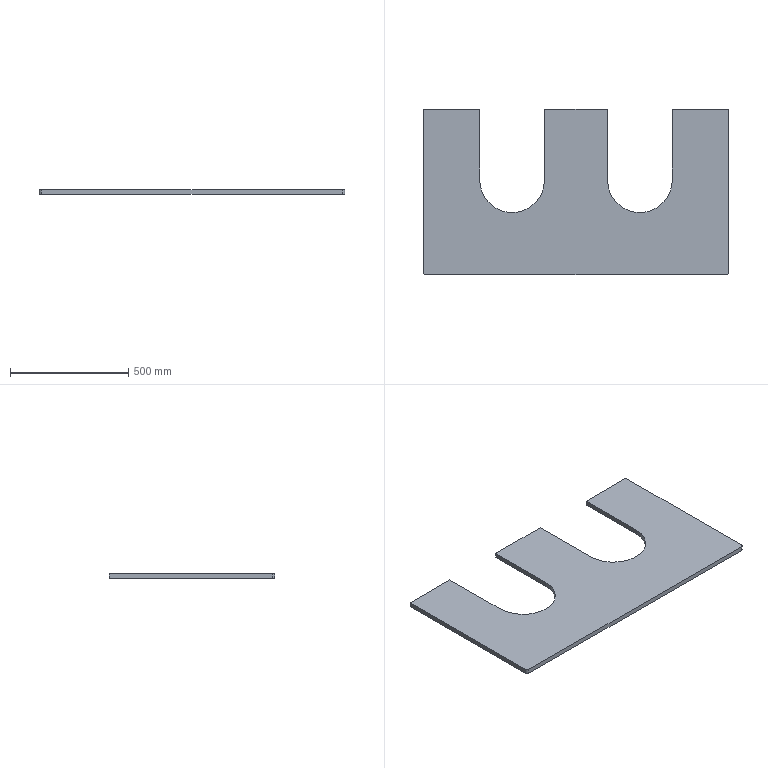Part | SolidWorks | features Extrusion 1, Fillet 1, ICE 1 | 1 solid | 16 faces | box 1290 x 700 x 20 mm | volume 13591851 mm3 | plane 12 | cylinder 4 | commonest cylinder face diameters 20 x2 274 x2
STEP:
#1=CARTESIAN_POINT('',(-407.,350.,20.));
#2=VERTEX_POINT('',#1);
#3=CARTESIAN_POINT('',(-645.,350.,20.));
#4=VERTEX_POINT('',#3);
#5=CARTESIAN_POINT('',(645.,350.,20.));
#6=DIRECTION('',(-1.,0.,0.));
#7=VECTOR('',#6,1000.);
#8=LINE('',#5,#7);
#9=EDGE_CURVE('',#2,#4,#8,.T.);
#10=ORIENTED_EDGE('',*,*,#9,.F.);
#11=CARTESIAN_POINT('',(-407.,350.,0.));
#12=VERTEX_POINT('',#11);
#13=CARTESIAN_POINT('',(-407.,350.,0.));
#14=DIRECTION('',(0.,0.,1.));
#15=VECTOR('',#14,1000.);
#16=LINE('',#13,#15);
#17=EDGE_CURVE('',#12,#2,#16,.T.);
#18=ORIENTED_EDGE('',*,*,#17,.F.);
#19=CARTESIAN_POINT('',(-645.,350.,0.));
#20=VERTEX_POINT('',#19);
#21=CARTESIAN_POINT('',(645.,350.,0.));
#22=DIRECTION('',(-1.,0.,0.));
#23=VECTOR('',#22,1000.);
#24=LINE('',#21,#23);
#25=EDGE_CURVE('',#12,#20,#24,.T.);
#26=ORIENTED_EDGE('',*,*,#25,.T.);
#27=CARTESIAN_POINT('',(-645.,350.,20.));
#28=DIRECTION('',(0.,0.,-1.));
#29=VECTOR('',#28,1000.);
#30=LINE('',#27,#29);
#31=EDGE_CURVE('',#4,#20,#30,.T.);
#32=ORIENTED_EDGE('',*,*,#31,.F.);
#33=EDGE_LOOP('',(#10,#18,#26,#32));
#34=FACE_OUTER_BOUND('',#33,.T.);
#35=CARTESIAN_POINT('',(645.,350.,20.));
#36=DIRECTION('',(0.,-1.,0.));
#37=DIRECTION('',(0.,0.,-1.));
#38=AXIS2_PLACEMENT_3D('',#35,#36,#37);
#39=PLANE('',#38);
#40=ADVANCED_FACE('',(#34),#39,.F.);
#41=CARTESIAN_POINT('',(133.,350.,0.));
#42=VERTEX_POINT('',#41);
#43=CARTESIAN_POINT('',(-133.,350.,0.));
#44=VERTEX_POINT('',#43);
#45=CARTESIAN_POINT('',(645.,350.,0.));
#46=DIRECTION('',(-1.,0.,0.));
#47=VECTOR('',#46,1000.);
#48=LINE('',#45,#47);
#49=EDGE_CURVE('',#42,#44,#48,.T.);
#50=ORIENTED_EDGE('',*,*,#49,.T.);
#51=CARTESIAN_POINT('',(-133.,350.,20.));
#52=VERTEX_POINT('',#51);
#53=CARTESIAN_POINT('',(-133.,350.,0.));
#54=DIRECTION('',(0.,0.,1.));
#55=VECTOR('',#54,1000.);
#56=LINE('',#53,#55);
#57=EDGE_CURVE('',#44,#52,#56,.T.);
#58=ORIENTED_EDGE('',*,*,#57,.T.);
#59=CARTESIAN_POINT('',(133.,350.,20.));
#60=VERTEX_POINT('',#59);
#61=CARTESIAN_POINT('',(645.,350.,20.));
#62=DIRECTION('',(-1.,0.,0.));
#63=VECTOR('',#62,1000.);
#64=LINE('',#61,#63);
#65=EDGE_CURVE('',#60,#52,#64,.T.);
#66=ORIENTED_EDGE('',*,*,#65,.F.);
#67=CARTESIAN_POINT('',(133.,350.,0.));
#68=DIRECTION('',(0.,0.,1.));
#69=VECTOR('',#68,1000.);
#70=LINE('',#67,#69);
#71=EDGE_CURVE('',#42,#60,#70,.T.);
#72=ORIENTED_EDGE('',*,*,#71,.F.);
#73=EDGE_LOOP('',(#50,#58,#66,#72));
#74=FACE_OUTER_BOUND('',#73,.T.);
#75=CARTESIAN_POINT('',(645.,350.,20.));
#76=DIRECTION('',(0.,-1.,0.));
#77=DIRECTION('',(0.,0.,-1.));
#78=AXIS2_PLACEMENT_3D('',#75,#76,#77);
#79=PLANE('',#78);
#80=ADVANCED_FACE('',(#74),#79,.F.);
#81=CARTESIAN_POINT('',(-645.,-340.,0.));
#82=VERTEX_POINT('',#81);
#83=CARTESIAN_POINT('',(-645.,-350.,0.));
#84=DIRECTION('',(0.,-1.,0.));
#85=VECTOR('',#84,1000.);
#86=LINE('',#83,#85);
#87=EDGE_CURVE('',#20,#82,#86,.T.);
#88=ORIENTED_EDGE('',*,*,#87,.T.);
#89=CARTESIAN_POINT('',(-645.,-340.,20.));
#90=VERTEX_POINT('',#89);
#91=CARTESIAN_POINT('',(-645.,-340.,20.));
#92=DIRECTION('',(0.,0.,1.));
#93=VECTOR('',#92,1000.);
#94=LINE('',#91,#93);
#95=EDGE_CURVE('',#82,#90,#94,.T.);
#96=ORIENTED_EDGE('',*,*,#95,.T.);
#97=CARTESIAN_POINT('',(-645.,-350.,20.));
#98=DIRECTION('',(0.,-1.,0.));
#99=VECTOR('',#98,1000.);
#100=LINE('',#97,#99);
#101=EDGE_CURVE('',#4,#90,#100,.T.);
#102=ORIENTED_EDGE('',*,*,#101,.F.);
#103=ORIENTED_EDGE('',*,*,#31,.T.);
#104=EDGE_LOOP('',(#88,#96,#102,#103));
#105=FACE_OUTER_BOUND('',#104,.T.);
#106=CARTESIAN_POINT('',(-645.,-350.,20.));
#107=DIRECTION('',(1.,0.,0.));
#108=DIRECTION('',(0.,0.,-1.));
#109=AXIS2_PLACEMENT_3D('',#106,#107,#108);
#110=PLANE('',#109);
#111=ADVANCED_FACE('',(#105),#110,.F.);
#112=CARTESIAN_POINT('',(-635.,-350.,0.));
#113=VERTEX_POINT('',#112);
#114=CARTESIAN_POINT('',(635.,-350.,0.));
#115=VERTEX_POINT('',#114);
#116=CARTESIAN_POINT('',(645.,-350.,0.));
#117=DIRECTION('',(1.,0.,0.));
#118=VECTOR('',#117,1000.);
#119=LINE('',#116,#118);
#120=EDGE_CURVE('',#113,#115,#119,.T.);
#121=ORIENTED_EDGE('',*,*,#120,.T.);
#122=CARTESIAN_POINT('',(635.,-350.,20.));
#123=VERTEX_POINT('',#122);
#124=CARTESIAN_POINT('',(635.,-350.,20.));
#125=DIRECTION('',(0.,0.,1.));
#126=VECTOR('',#125,1000.);
#127=LINE('',#124,#126);
#128=EDGE_CURVE('',#115,#123,#127,.T.);
#129=ORIENTED_EDGE('',*,*,#128,.T.);
#130=CARTESIAN_POINT('',(-635.,-350.,20.));
#131=VERTEX_POINT('',#130);
#132=CARTESIAN_POINT('',(645.,-350.,20.));
#133=DIRECTION('',(1.,0.,0.));
#134=VECTOR('',#133,1000.);
#135=LINE('',#132,#134);
#136=EDGE_CURVE('',#131,#123,#135,.T.);
#137=ORIENTED_EDGE('',*,*,#136,.F.);
#138=CARTESIAN_POINT('',(-635.,-350.,20.));
#139=DIRECTION('',(0.,0.,-1.));
#140=VECTOR('',#139,1000.);
#141=LINE('',#138,#140);
#142=EDGE_CURVE('',#131,#113,#141,.T.);
#143=ORIENTED_EDGE('',*,*,#142,.T.);
#144=EDGE_LOOP('',(#121,#129,#137,#143));
#145=FACE_OUTER_BOUND('',#144,.T.);
#146=CARTESIAN_POINT('',(645.,-350.,20.));
#147=DIRECTION('',(0.,1.,0.));
#148=DIRECTION('',(0.,0.,1.));
#149=AXIS2_PLACEMENT_3D('',#146,#147,#148);
#150=PLANE('',#149);
#151=ADVANCED_FACE('',(#145),#150,.F.);
#152=CARTESIAN_POINT('',(645.,-340.,20.));
#153=VERTEX_POINT('',#152);
#154=CARTESIAN_POINT('',(645.,350.,20.));
#155=VERTEX_POINT('',#154);
#156=CARTESIAN_POINT('',(645.,-350.,20.));
#157=DIRECTION('',(0.,1.,0.));
#158=VECTOR('',#157,1000.);
#159=LINE('',#156,#158);
#160=EDGE_CURVE('',#153,#155,#159,.T.);
#161=ORIENTED_EDGE('',*,*,#160,.F.);
#162=CARTESIAN_POINT('',(645.,-340.,0.));
#163=VERTEX_POINT('',#162);
#164=CARTESIAN_POINT('',(645.,-340.,20.));
#165=DIRECTION('',(0.,0.,-1.));
#166=VECTOR('',#165,1000.);
#167=LINE('',#164,#166);
#168=EDGE_CURVE('',#153,#163,#167,.T.);
#169=ORIENTED_EDGE('',*,*,#168,.T.);
#170=CARTESIAN_POINT('',(645.,350.,0.));
#171=VERTEX_POINT('',#170);
#172=CARTESIAN_POINT('',(645.,-350.,0.));
#173=DIRECTION('',(0.,1.,0.));
#174=VECTOR('',#173,1000.);
#175=LINE('',#172,#174);
#176=EDGE_CURVE('',#163,#171,#175,.T.);
#177=ORIENTED_EDGE('',*,*,#176,.T.);
#178=CARTESIAN_POINT('',(645.,350.,20.));
#179=DIRECTION('',(0.,0.,-1.));
#180=VECTOR('',#179,1000.);
#181=LINE('',#178,#180);
#182=EDGE_CURVE('',#155,#171,#181,.T.);
#183=ORIENTED_EDGE('',*,*,#182,.F.);
#184=EDGE_LOOP('',(#161,#169,#177,#183));
#185=FACE_OUTER_BOUND('',#184,.T.);
#186=CARTESIAN_POINT('',(645.,-350.,20.));
#187=DIRECTION('',(-1.,0.,0.));
#188=DIRECTION('',(0.,0.,1.));
#189=AXIS2_PLACEMENT_3D('',#186,#187,#188);
#190=PLANE('',#189);
#191=ADVANCED_FACE('',(#185),#190,.F.);
#192=CARTESIAN_POINT('',(407.,350.,0.));
#193=VERTEX_POINT('',#192);
#194=CARTESIAN_POINT('',(645.,350.,0.));
#195=DIRECTION('',(-1.,0.,0.));
#196=VECTOR('',#195,1000.);
#197=LINE('',#194,#196);
#198=EDGE_CURVE('',#171,#193,#197,.T.);
#199=ORIENTED_EDGE('',*,*,#198,.T.);
#200=CARTESIAN_POINT('',(407.,350.,20.));
#201=VERTEX_POINT('',#200);
#202=CARTESIAN_POINT('',(407.,350.,0.));
#203=DIRECTION('',(0.,0.,1.));
#204=VECTOR('',#203,1000.);
#205=LINE('',#202,#204);
#206=EDGE_CURVE('',#193,#201,#205,.T.);
#207=ORIENTED_EDGE('',*,*,#206,.T.);
#208=CARTESIAN_POINT('',(645.,350.,20.));
#209=DIRECTION('',(-1.,0.,0.));
#210=VECTOR('',#209,1000.);
#211=LINE('',#208,#210);
#212=EDGE_CURVE('',#155,#201,#211,.T.);
#213=ORIENTED_EDGE('',*,*,#212,.F.);
#214=ORIENTED_EDGE('',*,*,#182,.T.);
#215=EDGE_LOOP('',(#199,#207,#213,#214));
#216=FACE_OUTER_BOUND('',#215,.T.);
#217=CARTESIAN_POINT('',(645.,350.,20.));
#218=DIRECTION('',(0.,-1.,0.));
#219=DIRECTION('',(0.,0.,-1.));
#220=AXIS2_PLACEMENT_3D('',#217,#218,#219);
#221=PLANE('',#220);
#222=ADVANCED_FACE('',(#216),#221,.F.);
#223=ORIENTED_EDGE('',*,*,#136,.T.);
#224=CARTESIAN_POINT('',(635.,-340.,20.));
#225=DIRECTION('',(0.,0.,1.));
#226=DIRECTION('',(1.,0.,0.));
#227=AXIS2_PLACEMENT_3D('',#224,#225,#226);
#228=CIRCLE('',#227,10.);
#229=EDGE_CURVE('',#123,#153,#228,.T.);
#230=ORIENTED_EDGE('',*,*,#229,.T.);
#231=ORIENTED_EDGE('',*,*,#160,.T.);
#232=ORIENTED_EDGE('',*,*,#212,.T.);
#233=CARTESIAN_POINT('',(407.,50.,20.));
#234=VERTEX_POINT('',#233);
#235=CARTESIAN_POINT('',(407.,50.,20.));
#236=DIRECTION('',(0.,1.,0.));
#237=VECTOR('',#236,1000.);
#238=LINE('',#235,#237);
#239=EDGE_CURVE('',#234,#201,#238,.T.);
#240=ORIENTED_EDGE('',*,*,#239,.F.);
#241=CARTESIAN_POINT('',(133.,50.,20.));
#242=VERTEX_POINT('',#241);
#243=CARTESIAN_POINT('',(270.,50.,20.));
#244=DIRECTION('',(0.,0.,1.));
#245=DIRECTION('',(-1.,0.,0.));
#246=AXIS2_PLACEMENT_3D('',#243,#244,#245);
#247=CIRCLE('',#246,137.);
#248=EDGE_CURVE('',#242,#234,#247,.T.);
#249=ORIENTED_EDGE('',*,*,#248,.F.);
#250=CARTESIAN_POINT('',(133.,50.,20.));
#251=DIRECTION('',(0.,-1.,0.));
#252=VECTOR('',#251,1000.);
#253=LINE('',#250,#252);
#254=EDGE_CURVE('',#60,#242,#253,.T.);
#255=ORIENTED_EDGE('',*,*,#254,.F.);
#256=ORIENTED_EDGE('',*,*,#65,.T.);
#257=CARTESIAN_POINT('',(-133.,50.,20.));
#258=VERTEX_POINT('',#257);
#259=CARTESIAN_POINT('',(-133.,50.,20.));
#260=DIRECTION('',(0.,1.,0.));
#261=VECTOR('',#260,1000.);
#262=LINE('',#259,#261);
#263=EDGE_CURVE('',#258,#52,#262,.T.);
#264=ORIENTED_EDGE('',*,*,#263,.F.);
#265=CARTESIAN_POINT('',(-407.,50.,20.));
#266=VERTEX_POINT('',#265);
#267=CARTESIAN_POINT('',(-270.,50.,20.));
#268=DIRECTION('',(0.,0.,1.));
#269=DIRECTION('',(1.,0.,0.));
#270=AXIS2_PLACEMENT_3D('',#267,#268,#269);
#271=CIRCLE('',#270,137.);
#272=EDGE_CURVE('',#266,#258,#271,.T.);
#273=ORIENTED_EDGE('',*,*,#272,.F.);
#274=CARTESIAN_POINT('',(-407.,50.,20.));
#275=DIRECTION('',(0.,-1.,0.));
#276=VECTOR('',#275,1000.);
#277=LINE('',#274,#276);
#278=EDGE_CURVE('',#2,#266,#277,.T.);
#279=ORIENTED_EDGE('',*,*,#278,.F.);
#280=ORIENTED_EDGE('',*,*,#9,.T.);
#281=ORIENTED_EDGE('',*,*,#101,.T.);
#282=CARTESIAN_POINT('',(-635.,-340.,20.));
#283=DIRECTION('',(0.,0.,1.));
#284=DIRECTION('',(1.,0.,0.));
#285=AXIS2_PLACEMENT_3D('',#282,#283,#284);
#286=CIRCLE('',#285,10.);
#287=EDGE_CURVE('',#90,#131,#286,.T.);
#288=ORIENTED_EDGE('',*,*,#287,.T.);
#289=EDGE_LOOP('',(#223,#230,#231,#232,#240,#249,#255,#256,#264,#273,#279,#280,#281,#288));
#290=FACE_OUTER_BOUND('',#289,.T.);
#291=CARTESIAN_POINT('',(0.,0.,20.));
#292=DIRECTION('',(0.,0.,1.));
#293=DIRECTION('',(1.,0.,0.));
#294=AXIS2_PLACEMENT_3D('',#291,#292,#293);
#295=PLANE('',#294);
#296=ADVANCED_FACE('',(#290),#295,.T.);
#297=ORIENTED_EDGE('',*,*,#176,.F.);
#298=CARTESIAN_POINT('',(635.,-340.,0.));
#299=DIRECTION('',(0.,0.,-1.));
#300=DIRECTION('',(1.,0.,0.));
#301=AXIS2_PLACEMENT_3D('',#298,#299,#300);
#302=CIRCLE('',#301,10.);
#303=EDGE_CURVE('',#163,#115,#302,.T.);
#304=ORIENTED_EDGE('',*,*,#303,.T.);
#305=ORIENTED_EDGE('',*,*,#120,.F.);
#306=CARTESIAN_POINT('',(-635.,-340.,0.));
#307=DIRECTION('',(0.,0.,-1.));
#308=DIRECTION('',(1.,0.,0.));
#309=AXIS2_PLACEMENT_3D('',#306,#307,#308);
#310=CIRCLE('',#309,10.);
#311=EDGE_CURVE('',#113,#82,#310,.T.);
#312=ORIENTED_EDGE('',*,*,#311,.T.);
#313=ORIENTED_EDGE('',*,*,#87,.F.);
#314=ORIENTED_EDGE('',*,*,#25,.F.);
#315=CARTESIAN_POINT('',(-407.,50.,0.));
#316=VERTEX_POINT('',#315);
#317=CARTESIAN_POINT('',(-407.,50.,0.));
#318=DIRECTION('',(0.,-1.,0.));
#319=VECTOR('',#318,1000.);
#320=LINE('',#317,#319);
#321=EDGE_CURVE('',#12,#316,#320,.T.);
#322=ORIENTED_EDGE('',*,*,#321,.T.);
#323=CARTESIAN_POINT('',(-133.,50.,0.));
#324=VERTEX_POINT('',#323);
#325=CARTESIAN_POINT('',(-270.,50.,0.));
#326=DIRECTION('',(0.,0.,1.));
#327=DIRECTION('',(1.,0.,0.));
#328=AXIS2_PLACEMENT_3D('',#325,#326,#327);
#329=CIRCLE('',#328,137.);
#330=EDGE_CURVE('',#316,#324,#329,.T.);
#331=ORIENTED_EDGE('',*,*,#330,.T.);
#332=CARTESIAN_POINT('',(-133.,50.,0.));
#333=DIRECTION('',(0.,1.,0.));
#334=VECTOR('',#333,1000.);
#335=LINE('',#332,#334);
#336=EDGE_CURVE('',#324,#44,#335,.T.);
#337=ORIENTED_EDGE('',*,*,#336,.T.);
#338=ORIENTED_EDGE('',*,*,#49,.F.);
#339=CARTESIAN_POINT('',(133.,50.,0.));
#340=VERTEX_POINT('',#339);
#341=CARTESIAN_POINT('',(133.,50.,0.));
#342=DIRECTION('',(0.,-1.,0.));
#343=VECTOR('',#342,1000.);
#344=LINE('',#341,#343);
#345=EDGE_CURVE('',#42,#340,#344,.T.);
#346=ORIENTED_EDGE('',*,*,#345,.T.);
#347=CARTESIAN_POINT('',(407.,50.,0.));
#348=VERTEX_POINT('',#347);
#349=CARTESIAN_POINT('',(270.,50.,0.));
#350=DIRECTION('',(0.,0.,1.));
#351=DIRECTION('',(-1.,0.,0.));
#352=AXIS2_PLACEMENT_3D('',#349,#350,#351);
#353=CIRCLE('',#352,137.);
#354=EDGE_CURVE('',#340,#348,#353,.T.);
#355=ORIENTED_EDGE('',*,*,#354,.T.);
#356=CARTESIAN_POINT('',(407.,50.,0.));
#357=DIRECTION('',(0.,1.,0.));
#358=VECTOR('',#357,1000.);
#359=LINE('',#356,#358);
#360=EDGE_CURVE('',#348,#193,#359,.T.);
#361=ORIENTED_EDGE('',*,*,#360,.T.);
#362=ORIENTED_EDGE('',*,*,#198,.F.);
#363=EDGE_LOOP('',(#297,#304,#305,#312,#313,#314,#322,#331,#337,#338,#346,#355,#361,#362));
#364=FACE_OUTER_BOUND('',#363,.T.);
#365=CARTESIAN_POINT('',(0.,0.,0.));
#366=DIRECTION('',(0.,0.,1.));
#367=DIRECTION('',(1.,0.,0.));
#368=AXIS2_PLACEMENT_3D('',#365,#366,#367);
#369=PLANE('',#368);
#370=ADVANCED_FACE('',(#364),#369,.F.);
#371=ORIENTED_EDGE('',*,*,#248,.T.);
#372=CARTESIAN_POINT('',(407.,50.,0.));
#373=DIRECTION('',(0.,0.,1.));
#374=VECTOR('',#373,1000.);
#375=LINE('',#372,#374);
#376=EDGE_CURVE('',#348,#234,#375,.T.);
#377=ORIENTED_EDGE('',*,*,#376,.F.);
#378=ORIENTED_EDGE('',*,*,#354,.F.);
#379=CARTESIAN_POINT('',(133.,50.,0.));
#380=DIRECTION('',(0.,0.,1.));
#381=VECTOR('',#380,1000.);
#382=LINE('',#379,#381);
#383=EDGE_CURVE('',#340,#242,#382,.T.);
#384=ORIENTED_EDGE('',*,*,#383,.T.);
#385=EDGE_LOOP('',(#371,#377,#378,#384));
#386=FACE_OUTER_BOUND('',#385,.T.);
#387=CARTESIAN_POINT('',(270.,50.,0.));
#388=DIRECTION('',(0.,0.,1.));
#389=DIRECTION('',(1.,0.,0.));
#390=AXIS2_PLACEMENT_3D('',#387,#388,#389);
#391=CYLINDRICAL_SURFACE('',#390,137.);
#392=ADVANCED_FACE('',(#386),#391,.F.);
#393=ORIENTED_EDGE('',*,*,#254,.T.);
#394=ORIENTED_EDGE('',*,*,#383,.F.);
#395=ORIENTED_EDGE('',*,*,#345,.F.);
#396=ORIENTED_EDGE('',*,*,#71,.T.);
#397=EDGE_LOOP('',(#393,#394,#395,#396));
#398=FACE_OUTER_BOUND('',#397,.T.);
#399=CARTESIAN_POINT('',(133.,50.,0.));
#400=DIRECTION('',(-1.,0.,0.));
#401=DIRECTION('',(0.,0.,1.));
#402=AXIS2_PLACEMENT_3D('',#399,#400,#401);
#403=PLANE('',#402);
#404=ADVANCED_FACE('',(#398),#403,.F.);
#405=ORIENTED_EDGE('',*,*,#239,.T.);
#406=ORIENTED_EDGE('',*,*,#206,.F.);
#407=ORIENTED_EDGE('',*,*,#360,.F.);
#408=ORIENTED_EDGE('',*,*,#376,.T.);
#409=EDGE_LOOP('',(#405,#406,#407,#408));
#410=FACE_OUTER_BOUND('',#409,.T.);
#411=CARTESIAN_POINT('',(407.,50.,0.));
#412=DIRECTION('',(1.,0.,0.));
#413=DIRECTION('',(0.,0.,-1.));
#414=AXIS2_PLACEMENT_3D('',#411,#412,#413);
#415=PLANE('',#414);
#416=ADVANCED_FACE('',(#410),#415,.F.);
#417=ORIENTED_EDGE('',*,*,#272,.T.);
#418=CARTESIAN_POINT('',(-133.,50.,0.));
#419=DIRECTION('',(0.,0.,1.));
#420=VECTOR('',#419,1000.);
#421=LINE('',#418,#420);
#422=EDGE_CURVE('',#324,#258,#421,.T.);
#423=ORIENTED_EDGE('',*,*,#422,.F.);
#424=ORIENTED_EDGE('',*,*,#330,.F.);
#425=CARTESIAN_POINT('',(-407.,50.,0.));
#426=DIRECTION('',(0.,0.,1.));
#427=VECTOR('',#426,1000.);
#428=LINE('',#425,#427);
#429=EDGE_CURVE('',#316,#266,#428,.T.);
#430=ORIENTED_EDGE('',*,*,#429,.T.);
#431=EDGE_LOOP('',(#417,#423,#424,#430));
#432=FACE_OUTER_BOUND('',#431,.T.);
#433=CARTESIAN_POINT('',(-270.,50.,0.));
#434=DIRECTION('',(0.,0.,1.));
#435=DIRECTION('',(1.,0.,0.));
#436=AXIS2_PLACEMENT_3D('',#433,#434,#435);
#437=CYLINDRICAL_SURFACE('',#436,137.);
#438=ADVANCED_FACE('',(#432),#437,.F.);
#439=ORIENTED_EDGE('',*,*,#278,.T.);
#440=ORIENTED_EDGE('',*,*,#429,.F.);
#441=ORIENTED_EDGE('',*,*,#321,.F.);
#442=ORIENTED_EDGE('',*,*,#17,.T.);
#443=EDGE_LOOP('',(#439,#440,#441,#442));
#444=FACE_OUTER_BOUND('',#443,.T.);
#445=CARTESIAN_POINT('',(-407.,50.,0.));
#446=DIRECTION('',(-1.,0.,0.));
#447=DIRECTION('',(0.,0.,1.));
#448=AXIS2_PLACEMENT_3D('',#445,#446,#447);
#449=PLANE('',#448);
#450=ADVANCED_FACE('',(#444),#449,.F.);
#451=ORIENTED_EDGE('',*,*,#263,.T.);
#452=ORIENTED_EDGE('',*,*,#57,.F.);
#453=ORIENTED_EDGE('',*,*,#336,.F.);
#454=ORIENTED_EDGE('',*,*,#422,.T.);
#455=EDGE_LOOP('',(#451,#452,#453,#454));
#456=FACE_OUTER_BOUND('',#455,.T.);
#457=CARTESIAN_POINT('',(-133.,50.,0.));
#458=DIRECTION('',(1.,0.,0.));
#459=DIRECTION('',(0.,0.,-1.));
#460=AXIS2_PLACEMENT_3D('',#457,#458,#459);
#461=PLANE('',#460);
#462=ADVANCED_FACE('',(#456),#461,.F.);
#463=ORIENTED_EDGE('',*,*,#229,.F.);
#464=ORIENTED_EDGE('',*,*,#128,.F.);
#465=ORIENTED_EDGE('',*,*,#303,.F.);
#466=ORIENTED_EDGE('',*,*,#168,.F.);
#467=EDGE_LOOP('',(#463,#464,#465,#466));
#468=FACE_OUTER_BOUND('',#467,.T.);
#469=CARTESIAN_POINT('',(635.,-340.,20.));
#470=DIRECTION('',(0.,0.,-1.));
#471=DIRECTION('',(-1.,0.,0.));
#472=AXIS2_PLACEMENT_3D('',#469,#470,#471);
#473=CYLINDRICAL_SURFACE('',#472,10.);
#474=ADVANCED_FACE('',(#468),#473,.T.);
#475=ORIENTED_EDGE('',*,*,#287,.F.);
#476=ORIENTED_EDGE('',*,*,#95,.F.);
#477=ORIENTED_EDGE('',*,*,#311,.F.);
#478=ORIENTED_EDGE('',*,*,#142,.F.);
#479=EDGE_LOOP('',(#475,#476,#477,#478));
#480=FACE_OUTER_BOUND('',#479,.T.);
#481=CARTESIAN_POINT('',(-635.,-340.,20.));
#482=DIRECTION('',(0.,0.,-1.));
#483=DIRECTION('',(-1.,0.,0.));
#484=AXIS2_PLACEMENT_3D('',#481,#482,#483);
#485=CYLINDRICAL_SURFACE('',#484,10.);
#486=ADVANCED_FACE('',(#480),#485,.T.);
#487=CLOSED_SHELL('',(#40,#80,#111,#151,#191,#222,#296,#370,#392,#404,#416,#438,#450,#462,#474,#486));
#488=MANIFOLD_SOLID_BREP('',#487);
#489=CARTESIAN_POINT('',(0.,0.,0.));
#490=DIRECTION('',(0.,0.,1.));
#491=DIRECTION('',(1.,0.,0.));
#492=AXIS2_PLACEMENT_3D('',#489,#490,#491);
#493=(LENGTH_UNIT()NAMED_UNIT(*)SI_UNIT(.MILLI.,.METRE.));
#494=UNCERTAINTY_MEASURE_WITH_UNIT(LENGTH_MEASURE(0.00001),#493,'','');
#495=(NAMED_UNIT(*)PLANE_ANGLE_UNIT()SI_UNIT($,.RADIAN.));
#496=(NAMED_UNIT(*)SI_UNIT($,.STERADIAN.)SOLID_ANGLE_UNIT());
#497=(GEOMETRIC_REPRESENTATION_CONTEXT(3)GLOBAL_UNCERTAINTY_ASSIGNED_CONTEXT((#494))GLOBAL_UNIT_ASSIGNED_CONTEXT((#493,#495,#496))REPRESENTATION_CONTEXT('',''));
#498=ADVANCED_BREP_SHAPE_REPRESENTATION('',(#488,#492),#497);